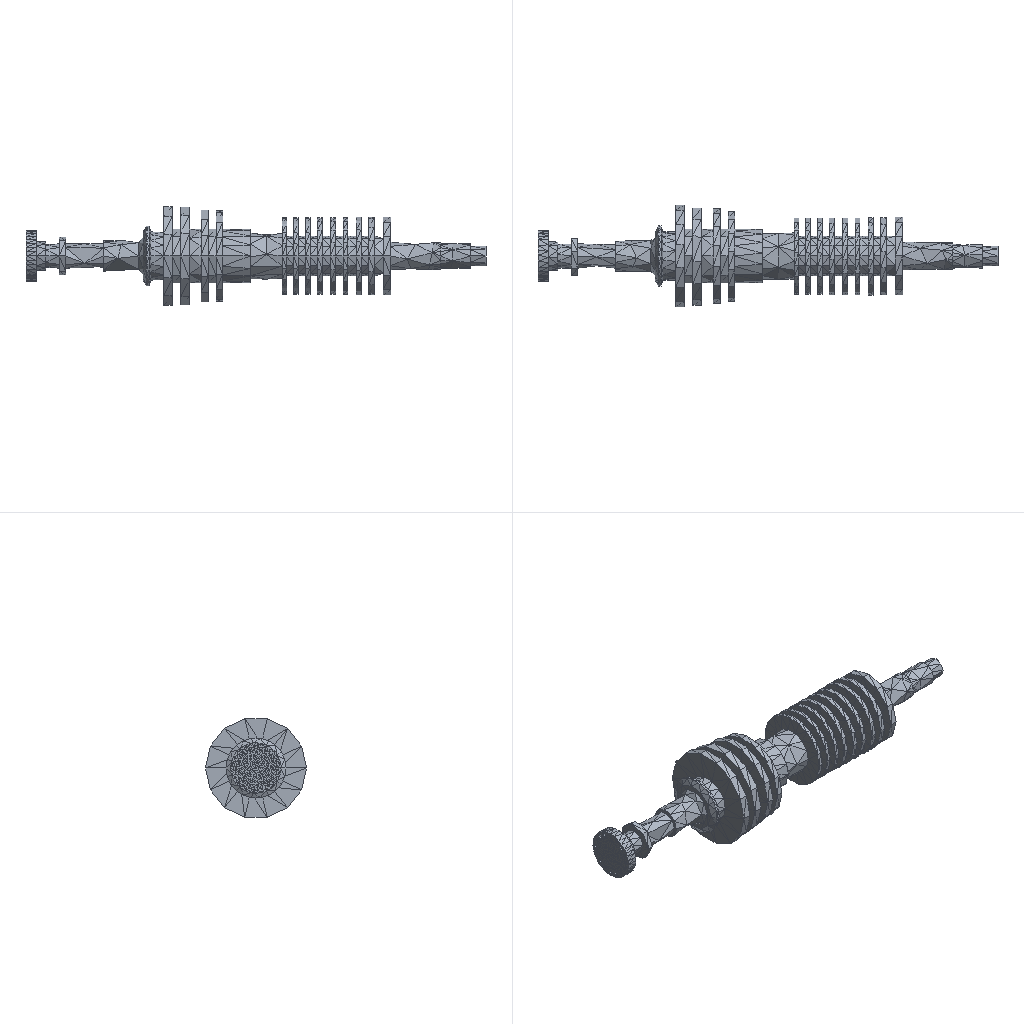Simulation study | ansys workbench
Ansys APDL input file, long lists of numbers shortened:
/batch
/config,noeldb,1     ! force off writing results to database
*get,_wallstrt,active,,time,wall
! ANSYS input file written by Workbench version 2022 R1
! File used for geometry attach:
/title,_______--__ (B5)
! ****** Begin Custom Load Command Snippet ******
/COM, ACT Extensions:
/COM,     LSDYNA, 2021.1
/COM,
! ****** End   Custom Load Command Snippet ******
*DIM,_wb_ProjectScratch_dir,string,248
_wb_ProjectScratch_dir(1) = ''
*DIM,_wb_SolverFiles_dir,string,248
_wb_SolverFiles_dir(1) = ''
*DIM,_wb_userfiles_dir,string,248
_wb_userfiles_dir(1) = ''
/com,--- Data in consistent NMM units. See Solving Units in the help system for more information.
/units,MPA
/nopr
/wb,file,start              !  signify a WB generated input file
/prep7
! Turn off shape checking because checks already performed inside WB mesher.
! See help system for more information.
SHPP,OFF,,NOWARN
/nolist
etcon,set             ! allow ANSYS to choose best KEYOP's for 180x elements, resets any applicable keyopt to MAPDL defaults
/com,*********** Nodes for the whole assembly ***********
nblock,3,,19310
(1i9,3e20.9e3)
        1     4.906201621E+04    -3.060000000E+02     1.550000000E+03
! (17554 more lines like these left out)
-1
/wb,elem,start            !  set before creation of elements
/com,*********** Elements for Body 1 "_____+115mm\_____" ***********
et,1,187
eblock,19,solid,,9763
(19i9)
        1        1        1        1        0        0        0        0       10        0        1     2257     2779     2330     2541    15734    16136    15725    15727
! (19525 more lines like these left out)
-1
/wb,elem,end               !  done creating elements
/com,*********** Send User Defined Coordinate System(s) ***********
csys,0
toffst,273.15,  ! Temperature offset from absolute zero
/com,*********** Set Reference Temperature ***********
tref,22.
/wb,mat,start              !  starting to send materials
/com,*********** Send Materials ***********
Temperature = 'TEMP' ! Temperature
MP,DENS,1,7.85e-09,	! tonne mm^-3
MP,ALPX,1,1.2e-05,	! C^-1
MP,C,1,434000000,	! mm^2 s^-2 C^-1
MP,KXX,1,60.5,	! tonne mm s^-3 C^-1
MP,RSVX,1,0.00017,	! ohm mm
MP,EX,1,200000,	! tonne s^-2 mm^-1
MP,NUXY,1,0.3,
MP,MURX,1,10000,
/wb,mat,end                !  done sending materials
!************************* Model Summary ********************
!_____+115mm\_____,	结构钢,	matid,	1
!************************* End Model Summary ********************
! get the diagonal of the bounding box. Needed later for other things
*get,_xmin,node,,mnloc,x
*get,_ymin,node,,mnloc,y
*get,_zmin,node,,mnloc,z
*get,_xmax,node,,mxloc,x
*get,_ymax,node,,mxloc,y
*get,_zmax,node,,mxloc,z
_ASMDIAG=(_xmax-_xmin)*(_xmax-_xmin)+(_ymax-_ymin)*(_ymax-_ymin)+(_zmax-_zmin)*(_zmax-_zmin)
_ASMDIAG=SQRT(_ASMDIAG)
/wb,contact,start          !  starting to send contact
/wb,contact,end            !  done creating contacts
/golist
/wb,load,start             !  starting to send loads
/gst,on,on
fini
*get,_numnode,node,0,count
*get,_numelem,elem,0,count
*get, _MAXELEMNUM, elem, 0, NUM, MAX
*get, _MAXNODENUM, node, 0, NUM, MAX
*get, _MAXELEMTYPE, etyp, 0, NUM, MAX
*get, _MAXREALCONST, real, 0, NUM, MAX
/go
/wb,load,end               !  done creating loads
/com,--- Number of total nodes = %_numnode%
/com,--- Number of contact elements = 0
/com,--- Number of spring elements = 0
/com,--- Number of bearing elements = 0
/com,--- Number of solid elements = 9763
/com,--- Number of condensed parts = 0
/com,--- Number of total elements = %_numelem%
*get,_wallbsol,active,,time,wall
/solu
antype,2                   ! modal analysis
_thickRatio=  1     ! Ratio of thick parts in the model
modopt,damp,12
outres,erase
outres,all,none
outres,nsol,all
outres,etmp,all
mxpand                    ! default expand in case of complex solution
dmpopt,esav,no
dmpopt,emat,no
dmpopt,full,no
! *********** WB SOLVE COMMAND ***********
! check interactive state
*get,ANSINTER_,active,,int
*if,ANSINTER_,ne,0,then
/eof
*endif
solve
/com *************** Write FE CONNECTORS *********
CEWRITE,file,ce,,INTE
*get,_nmodalsolproc,active,0,numcpu
fini
/nopr
*get,_numnode,node,0,count
*get,_numelem,elem,0,count
*get, _MAXELEMNUM, elem, 0, NUM, MAX
*get, _MAXNODENUM, node, 0, NUM, MAX,,,INTERNAL
*get, _MAXELEMTYPE, etyp, 0, NUM, MAX
*get, _MAXREALCONST, real, 0, NUM, MAX
/gopr
*get,_wallasol,active,,time,wall
/post1
/nopr
*dim,_direction,CHAR,6,1
_direction(1) = 'X'
_direction(2) = 'Y'
_direction(3) = 'Z'
_direction(4) = 'X'
_direction(5) = 'Y'
_direction(6) = 'Z'
*get,_lastLS,active,0,set,LSTP
*get,_beginset,active,0,set,nset,first,_lastLS
*get,_endset,active,0,set,nset,last,_lastLS
_nummodes = 0
*if,_endset,gt,0,then
_nummodes = _endset - _beginset + 1
*endif
_nummodes=_nummodes/2
*do,i_mode,1,_nummodes
   *do,j_component,1,6
		*if,j_component,gt,3,then
			*get,PFACT_%i_mode%_%j_component%,MODE,%i_mode%,PFACT,IMAG,DIREC,_direction(%j_component%)
		*else
			*get,PFACT_%i_mode%_%j_component%,MODE,%i_mode%,PFACT,,DIREC,_direction(%j_component%)
		*endif
   *enddo
*enddo
*dim,_tmdirection,CHAR,6,1
_tmdirection(1) = 'X'
_tmdirection(2) = 'Y'
_tmdirection(3) = 'Z'
_tmdirection(4) = 'X'
_tmdirection(5) = 'Y'
_tmdirection(6) = 'Z'
*do,j_component,1,6
    *if,j_component,gt,3,then
        *get,TOTALMASS_%j_component%,ELEM,0,IOR,_tmdirection(%j_component%)
    *else
        *get,TOTALMASS_%j_component%,ELEM,0,MTOT,_tmdirection(%j_component%)
    *endif
*enddo
/gopr
xmlo,ENCODING,ISO-8859-1
xmlo,parm
/xml,parm,xml
fini
/gopr
*get,_walldone,active,,time,wall
_preptime=(_wallbsol-_wallstrt)*3600
_solvtime=(_wallasol-_wallbsol)*3600
_posttime=(_walldone-_wallasol)*3600
_totaltim=(_walldone-_wallstrt)*3600
*get,_dlbratio,active,0,solu,dlbr
*get,_combtime,active,0,solu,comb
*get,_ssmode,active,0,solu,ssmm
*get,_ndofs,active,0,solu,ndof
/fclean				!clean distributed files
/com,--- Total number of nodes = %_numnode%
/com,--- Total number of elements = %_numelem%
/com,--- Element load balance ratio = %_dlbratio%
/com,--- Time to combine distributed files = %_combtime%
/com,--- Sparse memory mode = %_ssmode%
/com,--- Number of DOF = %_ndofs%
/wb,file,end               ! done with WB generated input